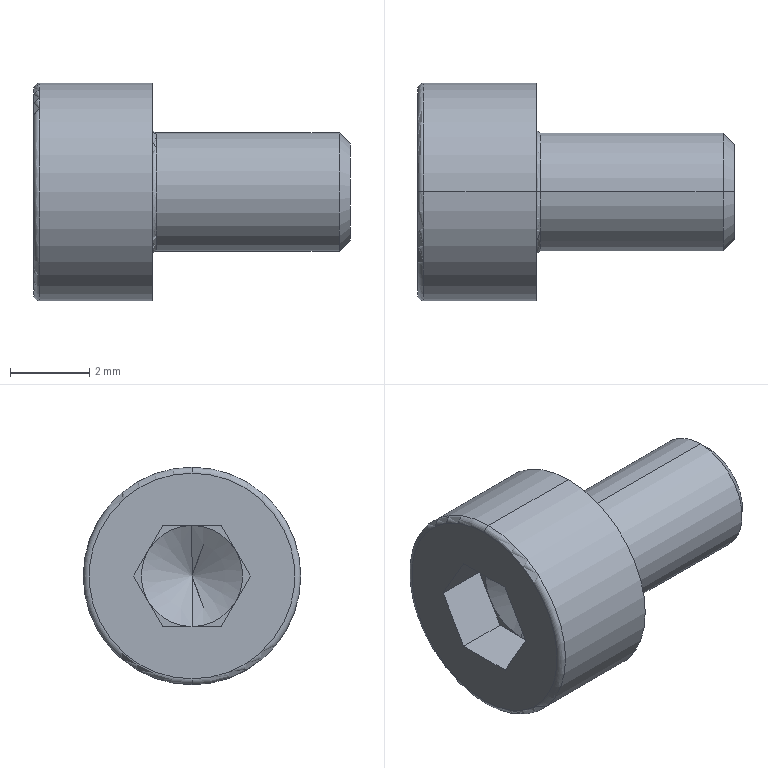Part | NX | 1 solid | 27 faces | box 8 x 5.5 x 5.5 mm | volume 97.562 mm3 | plane 15 | cone 4 | torus 4 | cylinder 4 | commonest cylinder face diameters 3 x2 5.5 x2
STEP:
#1=CARTESIAN_POINT('',(2.039,0.,0.));
#2=VERTEX_POINT('',#1);
#3=CARTESIAN_POINT('',(1.3,0.,1.28));
#4=VERTEX_POINT('',#3);
#5=CARTESIAN_POINT('',(1.3,0.,1.28));
#6=DIRECTION('',(-0.5,0.,0.866));
#7=VECTOR('',#6,1.);
#8=LINE('',#5,#7);
#9=EDGE_CURVE('',#2,#4,#8,.T.);
#10=ORIENTED_EDGE('',*,*,#9,.F.);
#11=CARTESIAN_POINT('',(1.3,0.,-1.28));
#12=VERTEX_POINT('',#11);
#13=CARTESIAN_POINT('',(1.3,0.,-1.28));
#14=DIRECTION('',(-0.5,0.,-0.866));
#15=VECTOR('',#14,1.);
#16=LINE('',#13,#15);
#17=EDGE_CURVE('',#2,#12,#16,.T.);
#18=ORIENTED_EDGE('',*,*,#17,.T.);
#19=CARTESIAN_POINT('',(1.3,-1.109,-0.64));
#20=VERTEX_POINT('',#19);
#21=CARTESIAN_POINT('',(1.3,0.,0.));
#22=DIRECTION('',(-1.,0.,0.));
#23=DIRECTION('',(0.,0.,1.));
#24=AXIS2_PLACEMENT_3D('',#21,#22,#23);
#25=CIRCLE('',#24,1.28);
#26=EDGE_CURVE('',#12,#20,#25,.T.);
#27=ORIENTED_EDGE('',*,*,#26,.T.);
#28=CARTESIAN_POINT('',(1.3,-1.109,0.64));
#29=VERTEX_POINT('',#28);
#30=CARTESIAN_POINT('',(1.3,0.,0.));
#31=DIRECTION('',(-1.,0.,0.));
#32=DIRECTION('',(0.,0.,1.));
#33=AXIS2_PLACEMENT_3D('',#30,#31,#32);
#34=CIRCLE('',#33,1.28);
#35=EDGE_CURVE('',#20,#29,#34,.T.);
#36=ORIENTED_EDGE('',*,*,#35,.T.);
#37=CARTESIAN_POINT('',(1.3,0.,0.));
#38=DIRECTION('',(-1.,0.,0.));
#39=DIRECTION('',(0.,0.,1.));
#40=AXIS2_PLACEMENT_3D('',#37,#38,#39);
#41=CIRCLE('',#40,1.28);
#42=EDGE_CURVE('',#29,#4,#41,.T.);
#43=ORIENTED_EDGE('',*,*,#42,.T.);
#44=EDGE_LOOP('',(#10,#18,#27,#36,#43));
#45=FACE_OUTER_BOUND('',#44,.T.);
#46=CARTESIAN_POINT('',(1.3,0.,0.));
#47=DIRECTION('',(-1.,0.,0.));
#48=DIRECTION('',(0.,0.,1.));
#49=AXIS2_PLACEMENT_3D('',#46,#47,#48);
#50=CONICAL_SURFACE('',#49,1.28,60.);
#51=ADVANCED_FACE('',(#45),#50,.F.);
#52=CARTESIAN_POINT('',(0.15,0.,-2.75));
#53=VERTEX_POINT('',#52);
#54=CARTESIAN_POINT('',(0.15,0.,2.75));
#55=VERTEX_POINT('',#54);
#56=CARTESIAN_POINT('',(0.15,0.,0.));
#57=DIRECTION('',(1.,0.,0.));
#58=DIRECTION('',(0.,0.,1.));
#59=AXIS2_PLACEMENT_3D('',#56,#57,#58);
#60=CIRCLE('',#59,2.75);
#61=EDGE_CURVE('',#53,#55,#60,.T.);
#62=ORIENTED_EDGE('',*,*,#61,.F.);
#63=CARTESIAN_POINT('',(0.,0.,-2.6));
#64=VERTEX_POINT('',#63);
#65=CARTESIAN_POINT('',(0.15,0.,-2.6));
#66=DIRECTION('',(0.,1.,0.));
#67=DIRECTION('',(0.,0.,1.));
#68=AXIS2_PLACEMENT_3D('',#65,#66,#67);
#69=CIRCLE('',#68,0.15);
#70=EDGE_CURVE('',#53,#64,#69,.T.);
#71=ORIENTED_EDGE('',*,*,#70,.T.);
#72=CARTESIAN_POINT('',(0.,0.,2.6));
#73=VERTEX_POINT('',#72);
#74=CARTESIAN_POINT('',(0.,0.,0.));
#75=DIRECTION('',(-1.,0.,0.));
#76=DIRECTION('',(0.,0.,1.));
#77=AXIS2_PLACEMENT_3D('',#74,#75,#76);
#78=CIRCLE('',#77,2.6);
#79=EDGE_CURVE('',#73,#64,#78,.T.);
#80=ORIENTED_EDGE('',*,*,#79,.F.);
#81=CARTESIAN_POINT('',(0.15,0.,2.6));
#82=DIRECTION('',(0.,-1.,0.));
#83=DIRECTION('',(0.,0.,-1.));
#84=AXIS2_PLACEMENT_3D('',#81,#82,#83);
#85=CIRCLE('',#84,0.15);
#86=EDGE_CURVE('',#55,#73,#85,.T.);
#87=ORIENTED_EDGE('',*,*,#86,.F.);
#88=EDGE_LOOP('',(#62,#71,#80,#87));
#89=FACE_OUTER_BOUND('',#88,.T.);
#90=CARTESIAN_POINT('',(0.15,0.,0.));
#91=DIRECTION('',(-1.,0.,0.));
#92=DIRECTION('',(0.,0.,1.));
#93=AXIS2_PLACEMENT_3D('',#90,#91,#92);
#94=TOROIDAL_SURFACE('',#93,2.6,0.15);
#95=ADVANCED_FACE('',(#89),#94,.T.);
#96=CARTESIAN_POINT('',(3.1,0.,1.5));
#97=VERTEX_POINT('',#96);
#98=CARTESIAN_POINT('',(3.1,0.,-1.5));
#99=VERTEX_POINT('',#98);
#100=CARTESIAN_POINT('',(3.1,0.,0.));
#101=DIRECTION('',(1.,0.,0.));
#102=DIRECTION('',(0.,0.,-1.));
#103=AXIS2_PLACEMENT_3D('',#100,#101,#102);
#104=CIRCLE('',#103,1.5);
#105=EDGE_CURVE('',#97,#99,#104,.T.);
#106=ORIENTED_EDGE('',*,*,#105,.F.);
#107=CARTESIAN_POINT('',(3.,0.,1.6));
#108=VERTEX_POINT('',#107);
#109=CARTESIAN_POINT('',(3.1,0.,1.6));
#110=DIRECTION('',(0.,-1.,0.));
#111=DIRECTION('',(0.,0.,1.));
#112=AXIS2_PLACEMENT_3D('',#109,#110,#111);
#113=CIRCLE('',#112,0.1);
#114=EDGE_CURVE('',#108,#97,#113,.T.);
#115=ORIENTED_EDGE('',*,*,#114,.F.);
#116=CARTESIAN_POINT('',(3.,0.,-1.6));
#117=VERTEX_POINT('',#116);
#118=CARTESIAN_POINT('',(3.,0.,0.));
#119=DIRECTION('',(-1.,0.,0.));
#120=DIRECTION('',(0.,0.,-1.));
#121=AXIS2_PLACEMENT_3D('',#118,#119,#120);
#122=CIRCLE('',#121,1.6);
#123=EDGE_CURVE('',#117,#108,#122,.T.);
#124=ORIENTED_EDGE('',*,*,#123,.F.);
#125=CARTESIAN_POINT('',(3.1,0.,-1.6));
#126=DIRECTION('',(0.,1.,0.));
#127=DIRECTION('',(0.,0.,-1.));
#128=AXIS2_PLACEMENT_3D('',#125,#126,#127);
#129=CIRCLE('',#128,0.1);
#130=EDGE_CURVE('',#117,#99,#129,.T.);
#131=ORIENTED_EDGE('',*,*,#130,.T.);
#132=EDGE_LOOP('',(#106,#115,#124,#131));
#133=FACE_OUTER_BOUND('',#132,.T.);
#134=CARTESIAN_POINT('',(3.1,0.,0.));
#135=DIRECTION('',(1.,0.,0.));
#136=DIRECTION('',(0.,0.,-1.));
#137=AXIS2_PLACEMENT_3D('',#134,#135,#136);
#138=TOROIDAL_SURFACE('',#137,1.6,0.1);
#139=ADVANCED_FACE('',(#133),#138,.F.);
#140=CARTESIAN_POINT('',(8.,0.,1.22));
#141=VERTEX_POINT('',#140);
#142=CARTESIAN_POINT('',(8.,0.,-1.22));
#143=VERTEX_POINT('',#142);
#144=CARTESIAN_POINT('',(8.,0.,0.));
#145=DIRECTION('',(-1.,0.,0.));
#146=DIRECTION('',(0.,0.,1.));
#147=AXIS2_PLACEMENT_3D('',#144,#145,#146);
#148=CIRCLE('',#147,1.22);
#149=EDGE_CURVE('',#141,#143,#148,.T.);
#150=ORIENTED_EDGE('',*,*,#149,.T.);
#151=CARTESIAN_POINT('',(7.72,0.,-1.5));
#152=VERTEX_POINT('',#151);
#153=CARTESIAN_POINT('',(8.,0.,-1.22));
#154=DIRECTION('',(-0.7071,0.,-0.7071));
#155=VECTOR('',#154,1.);
#156=LINE('',#153,#155);
#157=EDGE_CURVE('',#143,#152,#156,.T.);
#158=ORIENTED_EDGE('',*,*,#157,.T.);
#159=CARTESIAN_POINT('',(7.72,0.,1.5));
#160=VERTEX_POINT('',#159);
#161=CARTESIAN_POINT('',(7.72,0.,0.));
#162=DIRECTION('',(-1.,0.,0.));
#163=DIRECTION('',(0.,0.,1.));
#164=AXIS2_PLACEMENT_3D('',#161,#162,#163);
#165=CIRCLE('',#164,1.5);
#166=EDGE_CURVE('',#160,#152,#165,.T.);
#167=ORIENTED_EDGE('',*,*,#166,.F.);
#168=CARTESIAN_POINT('',(8.,0.,1.22));
#169=DIRECTION('',(-0.7071,0.,0.7071));
#170=VECTOR('',#169,1.);
#171=LINE('',#168,#170);
#172=EDGE_CURVE('',#141,#160,#171,.T.);
#173=ORIENTED_EDGE('',*,*,#172,.F.);
#174=EDGE_LOOP('',(#150,#158,#167,#173));
#175=FACE_OUTER_BOUND('',#174,.T.);
#176=CARTESIAN_POINT('',(8.,0.,0.));
#177=DIRECTION('',(-1.,0.,0.));
#178=DIRECTION('',(0.,0.,1.));
#179=AXIS2_PLACEMENT_3D('',#176,#177,#178);
#180=CONICAL_SURFACE('',#179,1.22,45.);
#181=ADVANCED_FACE('',(#175),#180,.T.);
#182=ORIENTED_EDGE('',*,*,#166,.T.);
#183=CARTESIAN_POINT('',(-31.75,0.,-1.5));
#184=DIRECTION('',(-1.,0.,0.));
#185=VECTOR('',#184,1.);
#186=LINE('',#183,#185);
#187=EDGE_CURVE('',#152,#99,#186,.T.);
#188=ORIENTED_EDGE('',*,*,#187,.T.);
#189=CARTESIAN_POINT('',(3.1,0.,0.));
#190=DIRECTION('',(1.,0.,0.));
#191=DIRECTION('',(0.,0.,-1.));
#192=AXIS2_PLACEMENT_3D('',#189,#190,#191);
#193=CIRCLE('',#192,1.5);
#194=EDGE_CURVE('',#99,#97,#193,.T.);
#195=ORIENTED_EDGE('',*,*,#194,.T.);
#196=CARTESIAN_POINT('',(-31.75,0.,1.5));
#197=DIRECTION('',(-1.,0.,0.));
#198=VECTOR('',#197,1.);
#199=LINE('',#196,#198);
#200=EDGE_CURVE('',#160,#97,#199,.T.);
#201=ORIENTED_EDGE('',*,*,#200,.F.);
#202=EDGE_LOOP('',(#182,#188,#195,#201));
#203=FACE_OUTER_BOUND('',#202,.T.);
#204=CARTESIAN_POINT('',(-31.75,0.,0.));
#205=DIRECTION('',(-1.,0.,0.));
#206=DIRECTION('',(0.,0.,1.));
#207=AXIS2_PLACEMENT_3D('',#204,#205,#206);
#208=CYLINDRICAL_SURFACE('',#207,1.5);
#209=ADVANCED_FACE('',(#203),#208,.T.);
#210=CARTESIAN_POINT('',(3.,0.,2.75));
#211=VERTEX_POINT('',#210);
#212=CARTESIAN_POINT('',(3.,0.,-2.75));
#213=VERTEX_POINT('',#212);
#214=CARTESIAN_POINT('',(3.,0.,0.));
#215=DIRECTION('',(-1.,0.,0.));
#216=DIRECTION('',(0.,0.,1.));
#217=AXIS2_PLACEMENT_3D('',#214,#215,#216);
#218=CIRCLE('',#217,2.75);
#219=EDGE_CURVE('',#211,#213,#218,.T.);
#220=ORIENTED_EDGE('',*,*,#219,.T.);
#221=CARTESIAN_POINT('',(-31.75,0.,-2.75));
#222=DIRECTION('',(-1.,0.,0.));
#223=VECTOR('',#222,1.);
#224=LINE('',#221,#223);
#225=EDGE_CURVE('',#213,#53,#224,.T.);
#226=ORIENTED_EDGE('',*,*,#225,.T.);
#227=ORIENTED_EDGE('',*,*,#61,.T.);
#228=CARTESIAN_POINT('',(-31.75,0.,2.75));
#229=DIRECTION('',(-1.,0.,0.));
#230=VECTOR('',#229,1.);
#231=LINE('',#228,#230);
#232=EDGE_CURVE('',#211,#55,#231,.T.);
#233=ORIENTED_EDGE('',*,*,#232,.F.);
#234=EDGE_LOOP('',(#220,#226,#227,#233));
#235=FACE_OUTER_BOUND('',#234,.T.);
#236=CARTESIAN_POINT('',(-31.75,0.,0.));
#237=DIRECTION('',(-1.,0.,0.));
#238=DIRECTION('',(0.,0.,1.));
#239=AXIS2_PLACEMENT_3D('',#236,#237,#238);
#240=CYLINDRICAL_SURFACE('',#239,2.75);
#241=ADVANCED_FACE('',(#235),#240,.T.);
#242=CARTESIAN_POINT('',(0.,1.478,0.));
#243=VERTEX_POINT('',#242);
#244=CARTESIAN_POINT('',(0.,0.739,1.28));
#245=VERTEX_POINT('',#244);
#246=CARTESIAN_POINT('',(0.,1.478,0.));
#247=DIRECTION('',(0.,-0.5,0.866));
#248=VECTOR('',#247,1.);
#249=LINE('',#246,#248);
#250=EDGE_CURVE('',#243,#245,#249,.T.);
#251=ORIENTED_EDGE('',*,*,#250,.T.);
#252=CARTESIAN_POINT('',(0.,-0.739,1.28));
#253=VERTEX_POINT('',#252);
#254=CARTESIAN_POINT('',(0.,-0.739,1.28));
#255=DIRECTION('',(0.,1.,0.));
#256=VECTOR('',#255,1.);
#257=LINE('',#254,#256);
#258=EDGE_CURVE('',#253,#245,#257,.T.);
#259=ORIENTED_EDGE('',*,*,#258,.F.);
#260=CARTESIAN_POINT('',(0.,-1.478,0.));
#261=VERTEX_POINT('',#260);
#262=CARTESIAN_POINT('',(0.,-0.739,1.28));
#263=DIRECTION('',(0.,-0.5,-0.866));
#264=VECTOR('',#263,1.);
#265=LINE('',#262,#264);
#266=EDGE_CURVE('',#253,#261,#265,.T.);
#267=ORIENTED_EDGE('',*,*,#266,.T.);
#268=CARTESIAN_POINT('',(0.,-0.739,-1.28));
#269=VERTEX_POINT('',#268);
#270=CARTESIAN_POINT('',(0.,-1.478,0.));
#271=DIRECTION('',(0.,0.5,-0.866));
#272=VECTOR('',#271,1.);
#273=LINE('',#270,#272);
#274=EDGE_CURVE('',#261,#269,#273,.T.);
#275=ORIENTED_EDGE('',*,*,#274,.T.);
#276=CARTESIAN_POINT('',(0.,0.739,-1.28));
#277=VERTEX_POINT('',#276);
#278=CARTESIAN_POINT('',(0.,0.739,-1.28));
#279=DIRECTION('',(0.,-1.,0.));
#280=VECTOR('',#279,1.);
#281=LINE('',#278,#280);
#282=EDGE_CURVE('',#277,#269,#281,.T.);
#283=ORIENTED_EDGE('',*,*,#282,.F.);
#284=CARTESIAN_POINT('',(0.,1.478,0.));
#285=DIRECTION('',(0.,-0.5,-0.866));
#286=VECTOR('',#285,1.);
#287=LINE('',#284,#286);
#288=EDGE_CURVE('',#243,#277,#287,.T.);
#289=ORIENTED_EDGE('',*,*,#288,.F.);
#290=EDGE_LOOP('',(#251,#259,#267,#275,#283,#289));
#291=FACE_BOUND('',#290,.T.);
#292=ORIENTED_EDGE('',*,*,#79,.T.);
#293=CARTESIAN_POINT('',(0.,0.,0.));
#294=DIRECTION('',(-1.,0.,0.));
#295=DIRECTION('',(0.,0.,1.));
#296=AXIS2_PLACEMENT_3D('',#293,#294,#295);
#297=CIRCLE('',#296,2.6);
#298=EDGE_CURVE('',#64,#73,#297,.T.);
#299=ORIENTED_EDGE('',*,*,#298,.T.);
#300=EDGE_LOOP('',(#292,#299));
#301=FACE_BOUND('',#300,.T.);
#302=CARTESIAN_POINT('',(0.,0.,0.));
#303=DIRECTION('',(-1.,0.,0.));
#304=DIRECTION('',(0.,0.,1.));
#305=AXIS2_PLACEMENT_3D('',#302,#303,#304);
#306=PLANE('',#305);
#307=ADVANCED_FACE('',(#291,#301),#306,.T.);
#308=ORIENTED_EDGE('',*,*,#225,.F.);
#309=CARTESIAN_POINT('',(3.,0.,0.));
#310=DIRECTION('',(-1.,0.,0.));
#311=DIRECTION('',(0.,0.,1.));
#312=AXIS2_PLACEMENT_3D('',#309,#310,#311);
#313=CIRCLE('',#312,2.75);
#314=EDGE_CURVE('',#213,#211,#313,.T.);
#315=ORIENTED_EDGE('',*,*,#314,.T.);
#316=ORIENTED_EDGE('',*,*,#232,.T.);
#317=CARTESIAN_POINT('',(0.15,0.,0.));
#318=DIRECTION('',(1.,0.,0.));
#319=DIRECTION('',(0.,0.,1.));
#320=AXIS2_PLACEMENT_3D('',#317,#318,#319);
#321=CIRCLE('',#320,2.75);
#322=EDGE_CURVE('',#55,#53,#321,.T.);
#323=ORIENTED_EDGE('',*,*,#322,.T.);
#324=EDGE_LOOP('',(#308,#315,#316,#323));
#325=FACE_OUTER_BOUND('',#324,.T.);
#326=CARTESIAN_POINT('',(-31.75,0.,0.));
#327=DIRECTION('',(-1.,0.,0.));
#328=DIRECTION('',(0.,0.,1.));
#329=AXIS2_PLACEMENT_3D('',#326,#327,#328);
#330=CYLINDRICAL_SURFACE('',#329,2.75);
#331=ADVANCED_FACE('',(#325),#330,.T.);
#332=ORIENTED_EDGE('',*,*,#123,.T.);
#333=CARTESIAN_POINT('',(3.,0.,0.));
#334=DIRECTION('',(-1.,0.,0.));
#335=DIRECTION('',(0.,0.,-1.));
#336=AXIS2_PLACEMENT_3D('',#333,#334,#335);
#337=CIRCLE('',#336,1.6);
#338=EDGE_CURVE('',#108,#117,#337,.T.);
#339=ORIENTED_EDGE('',*,*,#338,.T.);
#340=EDGE_LOOP('',(#332,#339));
#341=FACE_BOUND('',#340,.T.);
#342=ORIENTED_EDGE('',*,*,#219,.F.);
#343=ORIENTED_EDGE('',*,*,#314,.F.);
#344=EDGE_LOOP('',(#342,#343));
#345=FACE_BOUND('',#344,.T.);
#346=CARTESIAN_POINT('',(3.,2.75,0.));
#347=DIRECTION('',(1.,0.,0.));
#348=DIRECTION('',(0.,0.,-1.));
#349=AXIS2_PLACEMENT_3D('',#346,#347,#348);
#350=PLANE('',#349);
#351=ADVANCED_FACE('',(#341,#345),#350,.T.);
#352=ORIENTED_EDGE('',*,*,#187,.F.);
#353=CARTESIAN_POINT('',(7.72,0.,0.));
#354=DIRECTION('',(-1.,0.,0.));
#355=DIRECTION('',(0.,0.,1.));
#356=AXIS2_PLACEMENT_3D('',#353,#354,#355);
#357=CIRCLE('',#356,1.5);
#358=EDGE_CURVE('',#152,#160,#357,.T.);
#359=ORIENTED_EDGE('',*,*,#358,.T.);
#360=ORIENTED_EDGE('',*,*,#200,.T.);
#361=ORIENTED_EDGE('',*,*,#105,.T.);
#362=EDGE_LOOP('',(#352,#359,#360,#361));
#363=FACE_OUTER_BOUND('',#362,.T.);
#364=CARTESIAN_POINT('',(-31.75,0.,0.));
#365=DIRECTION('',(-1.,0.,0.));
#366=DIRECTION('',(0.,0.,1.));
#367=AXIS2_PLACEMENT_3D('',#364,#365,#366);
#368=CYLINDRICAL_SURFACE('',#367,1.5);
#369=ADVANCED_FACE('',(#363),#368,.T.);
#370=ORIENTED_EDGE('',*,*,#157,.F.);
#371=CARTESIAN_POINT('',(8.,0.,0.));
#372=DIRECTION('',(-1.,0.,0.));
#373=DIRECTION('',(0.,0.,1.));
#374=AXIS2_PLACEMENT_3D('',#371,#372,#373);
#375=CIRCLE('',#374,1.22);
#376=EDGE_CURVE('',#143,#141,#375,.T.);
#377=ORIENTED_EDGE('',*,*,#376,.T.);
#378=ORIENTED_EDGE('',*,*,#172,.T.);
#379=ORIENTED_EDGE('',*,*,#358,.F.);
#380=EDGE_LOOP('',(#370,#377,#378,#379));
#381=FACE_OUTER_BOUND('',#380,.T.);
#382=CARTESIAN_POINT('',(8.,0.,0.));
#383=DIRECTION('',(-1.,0.,0.));
#384=DIRECTION('',(0.,0.,1.));
#385=AXIS2_PLACEMENT_3D('',#382,#383,#384);
#386=CONICAL_SURFACE('',#385,1.22,45.);
#387=ADVANCED_FACE('',(#381),#386,.T.);
#388=ORIENTED_EDGE('',*,*,#149,.F.);
#389=ORIENTED_EDGE('',*,*,#376,.F.);
#390=EDGE_LOOP('',(#388,#389));
#391=FACE_OUTER_BOUND('',#390,.T.);
#392=CARTESIAN_POINT('',(8.,1.22,0.));
#393=DIRECTION('',(1.,0.,0.));
#394=DIRECTION('',(0.,0.,-1.));
#395=AXIS2_PLACEMENT_3D('',#392,#393,#394);
#396=PLANE('',#395);
#397=ADVANCED_FACE('',(#391),#396,.T.);
#398=ORIENTED_EDGE('',*,*,#114,.T.);
#399=ORIENTED_EDGE('',*,*,#194,.F.);
#400=ORIENTED_EDGE('',*,*,#130,.F.);
#401=ORIENTED_EDGE('',*,*,#338,.F.);
#402=EDGE_LOOP('',(#398,#399,#400,#401));
#403=FACE_OUTER_BOUND('',#402,.T.);
#404=CARTESIAN_POINT('',(3.1,0.,0.));
#405=DIRECTION('',(1.,0.,0.));
#406=DIRECTION('',(0.,0.,-1.));
#407=AXIS2_PLACEMENT_3D('',#404,#405,#406);
#408=TOROIDAL_SURFACE('',#407,1.6,0.1);
#409=ADVANCED_FACE('',(#403),#408,.F.);
#410=ORIENTED_EDGE('',*,*,#70,.F.);
#411=ORIENTED_EDGE('',*,*,#322,.F.);
#412=ORIENTED_EDGE('',*,*,#86,.T.);
#413=ORIENTED_EDGE('',*,*,#298,.F.);
#414=EDGE_LOOP('',(#410,#411,#412,#413));
#415=FACE_OUTER_BOUND('',#414,.T.);
#416=CARTESIAN_POINT('',(0.15,0.,0.));
#417=DIRECTION('',(-1.,0.,0.));
#418=DIRECTION('',(0.,0.,1.));
#419=AXIS2_PLACEMENT_3D('',#416,#417,#418);
#420=TOROIDAL_SURFACE('',#419,2.6,0.15);
#421=ADVANCED_FACE('',(#415),#420,.T.);
#422=ORIENTED_EDGE('',*,*,#250,.F.);
#423=CARTESIAN_POINT('',(1.3,1.478,0.));
#424=VERTEX_POINT('',#423);
#425=CARTESIAN_POINT('',(1.3,1.478,0.));
#426=DIRECTION('',(-1.,0.,0.));
#427=VECTOR('',#426,1.);
#428=LINE('',#425,#427);
#429=EDGE_CURVE('',#424,#243,#428,.T.);
#430=ORIENTED_EDGE('',*,*,#429,.F.);
#431=CARTESIAN_POINT('',(1.3,1.109,0.64));
#432=VERTEX_POINT('',#431);
#433=CARTESIAN_POINT('',(1.3,1.478,0.));
#434=DIRECTION('',(0.,-0.5,0.866));
#435=VECTOR('',#434,1.);
#436=LINE('',#433,#435);
#437=EDGE_CURVE('',#424,#432,#436,.T.);
#438=ORIENTED_EDGE('',*,*,#437,.T.);
#439=CARTESIAN_POINT('',(1.3,0.739,1.28));
#440=VERTEX_POINT('',#439);
#441=CARTESIAN_POINT('',(1.3,1.478,0.));
#442=DIRECTION('',(0.,-0.5,0.866));
#443=VECTOR('',#442,1.);
#444=LINE('',#441,#443);
#445=EDGE_CURVE('',#432,#440,#444,.T.);
#446=ORIENTED_EDGE('',*,*,#445,.T.);
#447=CARTESIAN_POINT('',(1.3,0.739,1.28));
#448=DIRECTION('',(-1.,0.,0.));
#449=VECTOR('',#448,1.);
#450=LINE('',#447,#449);
#451=EDGE_CURVE('',#440,#245,#450,.T.);
#452=ORIENTED_EDGE('',*,*,#451,.T.);
#453=EDGE_LOOP('',(#422,#430,#438,#446,#452));
#454=FACE_OUTER_BOUND('',#453,.T.);
#455=CARTESIAN_POINT('',(1.3,1.478,0.));
#456=DIRECTION('',(0.,-0.866,-0.5));
#457=DIRECTION('',(0.,0.5,-0.866));
#458=AXIS2_PLACEMENT_3D('',#455,#456,#457);
#459=PLANE('',#458);
#460=ADVANCED_FACE('',(#454),#459,.T.);
#461=ORIENTED_EDGE('',*,*,#258,.T.);
#462=ORIENTED_EDGE('',*,*,#451,.F.);
#463=CARTESIAN_POINT('',(1.3,-0.739,1.28));
#464=DIRECTION('',(0.,1.,0.));
#465=VECTOR('',#464,1.);
#466=LINE('',#463,#465);
#467=EDGE_CURVE('',#4,#440,#466,.T.);
#468=ORIENTED_EDGE('',*,*,#467,.F.);
#469=CARTESIAN_POINT('',(1.3,-0.739,1.28));
#470=VERTEX_POINT('',#469);
#471=CARTESIAN_POINT('',(1.3,-0.739,1.28));
#472=DIRECTION('',(0.,1.,0.));
#473=VECTOR('',#472,1.);
#474=LINE('',#471,#473);
#475=EDGE_CURVE('',#470,#4,#474,.T.);
#476=ORIENTED_EDGE('',*,*,#475,.F.);
#477=CARTESIAN_POINT('',(1.3,-0.739,1.28));
#478=DIRECTION('',(-1.,0.,0.));
#479=VECTOR('',#478,1.);
#480=LINE('',#477,#479);
#481=EDGE_CURVE('',#470,#253,#480,.T.);
#482=ORIENTED_EDGE('',*,*,#481,.T.);
#483=EDGE_LOOP('',(#461,#462,#468,#476,#482));
#484=FACE_OUTER_BOUND('',#483,.T.);
#485=CARTESIAN_POINT('',(1.3,-0.739,1.28));
#486=DIRECTION('',(0.,0.,1.));
#487=DIRECTION('',(0.,-1.,0.));
#488=AXIS2_PLACEMENT_3D('',#485,#486,#487);
#489=PLANE('',#488);
#490=ADVANCED_FACE('',(#484),#489,.F.);
#491=ORIENTED_EDGE('',*,*,#266,.F.);
#492=ORIENTED_EDGE('',*,*,#481,.F.);
#493=CARTESIAN_POINT('',(1.3,-0.739,1.28));
#494=DIRECTION('',(0.,-0.5,-0.866));
#495=VECTOR('',#494,1.);
#496=LINE('',#493,#495);
#497=EDGE_CURVE('',#470,#29,#496,.T.);
#498=ORIENTED_EDGE('',*,*,#497,.T.);
#499=CARTESIAN_POINT('',(1.3,-1.478,0.));
#500=VERTEX_POINT('',#499);
#501=CARTESIAN_POINT('',(1.3,-0.739,1.28));
#502=DIRECTION('',(0.,-0.5,-0.866));
#503=VECTOR('',#502,1.);
#504=LINE('',#501,#503);
#505=EDGE_CURVE('',#29,#500,#504,.T.);
#506=ORIENTED_EDGE('',*,*,#505,.T.);
#507=CARTESIAN_POINT('',(1.3,-1.478,0.));
#508=DIRECTION('',(-1.,0.,0.));
#509=VECTOR('',#508,1.);
#510=LINE('',#507,#509);
#511=EDGE_CURVE('',#500,#261,#510,.T.);
#512=ORIENTED_EDGE('',*,*,#511,.T.);
#513=EDGE_LOOP('',(#491,#492,#498,#506,#512));
#514=FACE_OUTER_BOUND('',#513,.T.);
#515=CARTESIAN_POINT('',(1.3,-0.739,1.28));
#516=DIRECTION('',(0.,0.866,-0.5));
#517=DIRECTION('',(0.,0.5,0.866));
#518=AXIS2_PLACEMENT_3D('',#515,#516,#517);
#519=PLANE('',#518);
#520=ADVANCED_FACE('',(#514),#519,.T.);
#521=ORIENTED_EDGE('',*,*,#274,.F.);
#522=ORIENTED_EDGE('',*,*,#511,.F.);
#523=CARTESIAN_POINT('',(1.3,-1.478,0.));
#524=DIRECTION('',(0.,0.5,-0.866));
#525=VECTOR('',#524,1.);
#526=LINE('',#523,#525);
#527=EDGE_CURVE('',#500,#20,#526,.T.);
#528=ORIENTED_EDGE('',*,*,#527,.T.);
#529=CARTESIAN_POINT('',(1.3,-0.739,-1.28));
#530=VERTEX_POINT('',#529);
#531=CARTESIAN_POINT('',(1.3,-1.478,0.));
#532=DIRECTION('',(0.,0.5,-0.866));
#533=VECTOR('',#532,1.);
#534=LINE('',#531,#533);
#535=EDGE_CURVE('',#20,#530,#534,.T.);
#536=ORIENTED_EDGE('',*,*,#535,.T.);
#537=CARTESIAN_POINT('',(1.3,-0.739,-1.28));
#538=DIRECTION('',(-1.,0.,0.));
#539=VECTOR('',#538,1.);
#540=LINE('',#537,#539);
#541=EDGE_CURVE('',#530,#269,#540,.T.);
#542=ORIENTED_EDGE('',*,*,#541,.T.);
#543=EDGE_LOOP('',(#521,#522,#528,#536,#542));
#544=FACE_OUTER_BOUND('',#543,.T.);
#545=CARTESIAN_POINT('',(1.3,-1.478,0.));
#546=DIRECTION('',(0.,0.866,0.5));
#547=DIRECTION('',(0.,-0.5,0.866));
#548=AXIS2_PLACEMENT_3D('',#545,#546,#547);
#549=PLANE('',#548);
#550=ADVANCED_FACE('',(#544),#549,.T.);
#551=ORIENTED_EDGE('',*,*,#282,.T.);
#552=ORIENTED_EDGE('',*,*,#541,.F.);
#553=CARTESIAN_POINT('',(1.3,0.739,-1.28));
#554=DIRECTION('',(0.,-1.,0.));
#555=VECTOR('',#554,1.);
#556=LINE('',#553,#555);
#557=EDGE_CURVE('',#12,#530,#556,.T.);
#558=ORIENTED_EDGE('',*,*,#557,.F.);
#559=CARTESIAN_POINT('',(1.3,0.739,-1.28));
#560=VERTEX_POINT('',#559);
#561=CARTESIAN_POINT('',(1.3,0.739,-1.28));
#562=DIRECTION('',(0.,-1.,0.));
#563=VECTOR('',#562,1.);
#564=LINE('',#561,#563);
#565=EDGE_CURVE('',#560,#12,#564,.T.);
#566=ORIENTED_EDGE('',*,*,#565,.F.);
#567=CARTESIAN_POINT('',(1.3,0.739,-1.28));
#568=DIRECTION('',(-1.,0.,0.));
#569=VECTOR('',#568,1.);
#570=LINE('',#567,#569);
#571=EDGE_CURVE('',#560,#277,#570,.T.);
#572=ORIENTED_EDGE('',*,*,#571,.T.);
#573=EDGE_LOOP('',(#551,#552,#558,#566,#572));
#574=FACE_OUTER_BOUND('',#573,.T.);
#575=CARTESIAN_POINT('',(1.3,0.739,-1.28));
#576=DIRECTION('',(0.,0.,-1.));
#577=DIRECTION('',(0.,1.,0.));
#578=AXIS2_PLACEMENT_3D('',#575,#576,#577);
#579=PLANE('',#578);
#580=ADVANCED_FACE('',(#574),#579,.F.);
#581=ORIENTED_EDGE('',*,*,#288,.T.);
#582=ORIENTED_EDGE('',*,*,#571,.F.);
#583=CARTESIAN_POINT('',(1.3,1.109,-0.64));
#584=VERTEX_POINT('',#583);
#585=CARTESIAN_POINT('',(1.3,1.478,0.));
#586=DIRECTION('',(0.,-0.5,-0.866));
#587=VECTOR('',#586,1.);
#588=LINE('',#585,#587);
#589=EDGE_CURVE('',#584,#560,#588,.T.);
#590=ORIENTED_EDGE('',*,*,#589,.F.);
#591=CARTESIAN_POINT('',(1.3,1.478,0.));
#592=DIRECTION('',(0.,-0.5,-0.866));
#593=VECTOR('',#592,1.);
#594=LINE('',#591,#593);
#595=EDGE_CURVE('',#424,#584,#594,.T.);
#596=ORIENTED_EDGE('',*,*,#595,.F.);
#597=ORIENTED_EDGE('',*,*,#429,.T.);
#598=EDGE_LOOP('',(#581,#582,#590,#596,#597));
#599=FACE_OUTER_BOUND('',#598,.T.);
#600=CARTESIAN_POINT('',(1.3,1.478,0.));
#601=DIRECTION('',(0.,0.866,-0.5));
#602=DIRECTION('',(0.,0.5,0.866));
#603=AXIS2_PLACEMENT_3D('',#600,#601,#602);
#604=PLANE('',#603);
#605=ADVANCED_FACE('',(#599),#604,.F.);
#606=ORIENTED_EDGE('',*,*,#557,.T.);
#607=ORIENTED_EDGE('',*,*,#535,.F.);
#608=ORIENTED_EDGE('',*,*,#26,.F.);
#609=EDGE_LOOP('',(#606,#607,#608));
#610=FACE_OUTER_BOUND('',#609,.T.);
#611=CARTESIAN_POINT('',(1.3,1.478,0.));
#612=DIRECTION('',(1.,0.,0.));
#613=DIRECTION('',(0.,0.,-1.));
#614=AXIS2_PLACEMENT_3D('',#611,#612,#613);
#615=PLANE('',#614);
#616=ADVANCED_FACE('',(#610),#615,.F.);
#617=ORIENTED_EDGE('',*,*,#527,.F.);
#618=ORIENTED_EDGE('',*,*,#505,.F.);
#619=ORIENTED_EDGE('',*,*,#35,.F.);
#620=EDGE_LOOP('',(#617,#618,#619));
#621=FACE_OUTER_BOUND('',#620,.T.);
#622=CARTESIAN_POINT('',(1.3,1.478,0.));
#623=DIRECTION('',(1.,0.,0.));
#624=DIRECTION('',(0.,0.,-1.));
#625=AXIS2_PLACEMENT_3D('',#622,#623,#624);
#626=PLANE('',#625);
#627=ADVANCED_FACE('',(#621),#626,.F.);
#628=ORIENTED_EDGE('',*,*,#497,.F.);
#629=ORIENTED_EDGE('',*,*,#475,.T.);
#630=ORIENTED_EDGE('',*,*,#42,.F.);
#631=EDGE_LOOP('',(#628,#629,#630));
#632=FACE_OUTER_BOUND('',#631,.T.);
#633=CARTESIAN_POINT('',(1.3,1.478,0.));
#634=DIRECTION('',(1.,0.,0.));
#635=DIRECTION('',(0.,0.,-1.));
#636=AXIS2_PLACEMENT_3D('',#633,#634,#635);
#637=PLANE('',#636);
#638=ADVANCED_FACE('',(#632),#637,.F.);
#639=ORIENTED_EDGE('',*,*,#467,.T.);
#640=ORIENTED_EDGE('',*,*,#445,.F.);
#641=CARTESIAN_POINT('',(1.3,0.,0.));
#642=DIRECTION('',(-1.,0.,0.));
#643=DIRECTION('',(0.,0.,1.));
#644=AXIS2_PLACEMENT_3D('',#641,#642,#643);
#645=CIRCLE('',#644,1.28);
#646=EDGE_CURVE('',#4,#432,#645,.T.);
#647=ORIENTED_EDGE('',*,*,#646,.F.);
#648=EDGE_LOOP('',(#639,#640,#647));
#649=FACE_OUTER_BOUND('',#648,.T.);
#650=CARTESIAN_POINT('',(1.3,1.478,0.));
#651=DIRECTION('',(1.,0.,0.));
#652=DIRECTION('',(0.,0.,-1.));
#653=AXIS2_PLACEMENT_3D('',#650,#651,#652);
#654=PLANE('',#653);
#655=ADVANCED_FACE('',(#649),#654,.F.);
#656=ORIENTED_EDGE('',*,*,#437,.F.);
#657=ORIENTED_EDGE('',*,*,#595,.T.);
#658=CARTESIAN_POINT('',(1.3,0.,0.));
#659=DIRECTION('',(-1.,0.,0.));
#660=DIRECTION('',(0.,0.,1.));
#661=AXIS2_PLACEMENT_3D('',#658,#659,#660);
#662=CIRCLE('',#661,1.28);
#663=EDGE_CURVE('',#432,#584,#662,.T.);
#664=ORIENTED_EDGE('',*,*,#663,.F.);
#665=EDGE_LOOP('',(#656,#657,#664));
#666=FACE_OUTER_BOUND('',#665,.T.);
#667=CARTESIAN_POINT('',(1.3,1.478,0.));
#668=DIRECTION('',(1.,0.,0.));
#669=DIRECTION('',(0.,0.,-1.));
#670=AXIS2_PLACEMENT_3D('',#667,#668,#669);
#671=PLANE('',#670);
#672=ADVANCED_FACE('',(#666),#671,.F.);
#673=ORIENTED_EDGE('',*,*,#589,.T.);
#674=ORIENTED_EDGE('',*,*,#565,.T.);
#675=CARTESIAN_POINT('',(1.3,0.,0.));
#676=DIRECTION('',(-1.,0.,0.));
#677=DIRECTION('',(0.,0.,1.));
#678=AXIS2_PLACEMENT_3D('',#675,#676,#677);
#679=CIRCLE('',#678,1.28);
#680=EDGE_CURVE('',#584,#12,#679,.T.);
#681=ORIENTED_EDGE('',*,*,#680,.F.);
#682=EDGE_LOOP('',(#673,#674,#681));
#683=FACE_OUTER_BOUND('',#682,.T.);
#684=CARTESIAN_POINT('',(1.3,1.478,0.));
#685=DIRECTION('',(1.,0.,0.));
#686=DIRECTION('',(0.,0.,-1.));
#687=AXIS2_PLACEMENT_3D('',#684,#685,#686);
#688=PLANE('',#687);
#689=ADVANCED_FACE('',(#683),#688,.F.);
#690=ORIENTED_EDGE('',*,*,#17,.F.);
#691=ORIENTED_EDGE('',*,*,#9,.T.);
#692=ORIENTED_EDGE('',*,*,#646,.T.);
#693=ORIENTED_EDGE('',*,*,#663,.T.);
#694=ORIENTED_EDGE('',*,*,#680,.T.);
#695=EDGE_LOOP('',(#690,#691,#692,#693,#694));
#696=FACE_OUTER_BOUND('',#695,.T.);
#697=CARTESIAN_POINT('',(1.3,0.,0.));
#698=DIRECTION('',(-1.,0.,0.));
#699=DIRECTION('',(0.,0.,1.));
#700=AXIS2_PLACEMENT_3D('',#697,#698,#699);
#701=CONICAL_SURFACE('',#700,1.28,60.);
#702=ADVANCED_FACE('',(#696),#701,.F.);
#703=CLOSED_SHELL('',(#51,#95,#139,#181,#209,#241,#307,#331,#351,#369,#387,#397,#409,#421,#460,#490,#520,#550,#580,#605,#616,#627,#638,#655,#672,#689,#702));
#704=MANIFOLD_SOLID_BREP('',#703);
#705=(LENGTH_UNIT()NAMED_UNIT(*)SI_UNIT(.MILLI.,.METRE.));
#706=UNCERTAINTY_MEASURE_WITH_UNIT(LENGTH_MEASURE(0.00002),#705,'','');
#707=(NAMED_UNIT(*)PLANE_ANGLE_UNIT()SI_UNIT($,.RADIAN.));
#708=PLANE_ANGLE_MEASURE_WITH_UNIT(PLANE_ANGLE_MEASURE(0.01745),#707);
#709=DIMENSIONAL_EXPONENTS(0.,0.,0.,0.,0.,0.,0.);
#710=(CONVERSION_BASED_UNIT('DEGREE',#708)NAMED_UNIT(#709)PLANE_ANGLE_UNIT());
#711=(NAMED_UNIT(*)SI_UNIT($,.STERADIAN.)SOLID_ANGLE_UNIT());
#712=(GEOMETRIC_REPRESENTATION_CONTEXT(3)GLOBAL_UNCERTAINTY_ASSIGNED_CONTEXT((#706))GLOBAL_UNIT_ASSIGNED_CONTEXT((#705,#710,#711))REPRESENTATION_CONTEXT('',''));
#713=ADVANCED_BREP_SHAPE_REPRESENTATION('',(#704),#712);